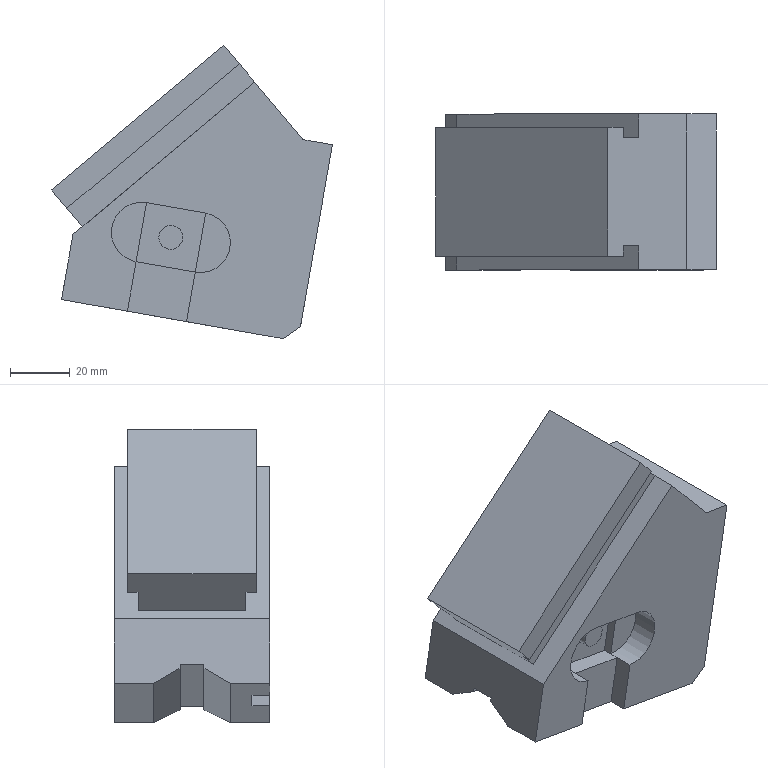Part | NX | features MAIN_BODY 2 | 1 solid | 38 faces | box 93.656 x 52 x 97.766 mm | volume 276638 mm3 | plane 35 | cylinder 2 | spline 1 | commonest cylinder face diameters 20 x2
STEP:
#1=CARTESIAN_POINT('',(264.879,130.,-23.774));
#2=VERTEX_POINT('',#1);
#3=CARTESIAN_POINT('',(297.078,130.,-29.451));
#4=VERTEX_POINT('',#3);
#5=CARTESIAN_POINT('',(223.218,130.,-16.428));
#6=DIRECTION('',(0.9848,0.,-0.1736));
#7=VECTOR('',#6,1000.);
#8=LINE('',#5,#7);
#9=EDGE_CURVE('',#2,#4,#8,.T.);
#10=ORIENTED_EDGE('',*,*,#9,.F.);
#11=CARTESIAN_POINT('',(264.879,136.,-23.774));
#12=VERTEX_POINT('',#11);
#13=CARTESIAN_POINT('',(264.879,182.,-23.774));
#14=DIRECTION('',(0.,-1.,0.));
#15=VECTOR('',#14,1000.);
#16=LINE('',#13,#15);
#17=EDGE_CURVE('',#12,#2,#16,.T.);
#18=ORIENTED_EDGE('',*,*,#17,.F.);
#19=CARTESIAN_POINT('',(245.183,136.,-20.301));
#20=VERTEX_POINT('',#19);
#21=CARTESIAN_POINT('',(223.218,136.,-16.428));
#22=DIRECTION('',(-0.9848,0.,0.1736));
#23=VECTOR('',#22,1000.);
#24=LINE('',#21,#23);
#25=EDGE_CURVE('',#12,#20,#24,.T.);
#26=ORIENTED_EDGE('',*,*,#25,.T.);
#27=CARTESIAN_POINT('',(245.183,130.,-20.301));
#28=VERTEX_POINT('',#27);
#29=CARTESIAN_POINT('',(245.183,182.,-20.301));
#30=DIRECTION('',(0.,-1.,0.));
#31=VECTOR('',#30,1000.);
#32=LINE('',#29,#31);
#33=EDGE_CURVE('',#20,#28,#32,.T.);
#34=ORIENTED_EDGE('',*,*,#33,.T.);
#35=CARTESIAN_POINT('',(223.218,130.,-16.428));
#36=VERTEX_POINT('',#35);
#37=CARTESIAN_POINT('',(223.218,130.,-16.428));
#38=DIRECTION('',(0.9848,0.,-0.1736));
#39=VECTOR('',#38,1000.);
#40=LINE('',#37,#39);
#41=EDGE_CURVE('',#36,#28,#40,.T.);
#42=ORIENTED_EDGE('',*,*,#41,.F.);
#43=CARTESIAN_POINT('',(223.218,143.01,-16.428));
#44=VERTEX_POINT('',#43);
#45=CARTESIAN_POINT('',(223.218,182.,-16.428));
#46=DIRECTION('',(0.,-1.,0.));
#47=VECTOR('',#46,1000.);
#48=LINE('',#45,#47);
#49=EDGE_CURVE('',#44,#36,#48,.T.);
#50=ORIENTED_EDGE('',*,*,#49,.F.);
#51=CARTESIAN_POINT('',(297.078,143.01,-29.451));
#52=VERTEX_POINT('',#51);
#53=CARTESIAN_POINT('',(223.218,143.01,-16.428));
#54=DIRECTION('',(-0.9848,0.,0.1736));
#55=VECTOR('',#54,1000.);
#56=LINE('',#53,#55);
#57=EDGE_CURVE('',#52,#44,#56,.T.);
#58=ORIENTED_EDGE('',*,*,#57,.F.);
#59=CARTESIAN_POINT('',(297.078,143.01,-29.451));
#60=DIRECTION('',(0.,1.,0.));
#61=VECTOR('',#60,1000.);
#62=LINE('',#59,#61);
#63=EDGE_CURVE('',#4,#52,#62,.T.);
#64=ORIENTED_EDGE('',*,*,#63,.F.);
#65=EDGE_LOOP('',(#10,#18,#26,#34,#42,#50,#58,#64));
#66=FACE_BOUND('',#65,.T.);
#67=CARTESIAN_POINT('',(223.218,182.,-16.428));
#68=DIRECTION('',(0.1736,0.,0.9848));
#69=DIRECTION('',(0.9848,0.,-0.1736));
#70=AXIS2_PLACEMENT_3D('',#67,#68,#69);
#71=PLANE('',#70);
#72=ADVANCED_FACE('',(#66),#71,.F.);
#73=CARTESIAN_POINT('',(313.55,130.,35.17));
#74=VERTEX_POINT('',#73);
#75=CARTESIAN_POINT('',(302.871,130.,-25.396));
#76=VERTEX_POINT('',#75);
#77=CARTESIAN_POINT('',(313.55,130.,35.17));
#78=DIRECTION('',(-0.1736,0.,-0.9848));
#79=VECTOR('',#78,1000.);
#80=LINE('',#77,#79);
#81=EDGE_CURVE('',#74,#76,#80,.T.);
#82=ORIENTED_EDGE('',*,*,#81,.F.);
#83=CARTESIAN_POINT('',(303.702,130.,36.906));
#84=VERTEX_POINT('',#83);
#85=CARTESIAN_POINT('',(303.702,130.,36.906));
#86=DIRECTION('',(0.9848,0.,-0.1736));
#87=VECTOR('',#86,1000.);
#88=LINE('',#85,#87);
#89=EDGE_CURVE('',#84,#74,#88,.T.);
#90=ORIENTED_EDGE('',*,*,#89,.F.);
#91=CARTESIAN_POINT('',(287.632,130.,56.058));
#92=VERTEX_POINT('',#91);
#93=CARTESIAN_POINT('',(287.632,130.,56.058));
#94=DIRECTION('',(0.6428,0.,-0.766));
#95=VECTOR('',#94,1000.);
#96=LINE('',#93,#95);
#97=EDGE_CURVE('',#92,#84,#96,.T.);
#98=ORIENTED_EDGE('',*,*,#97,.F.);
#99=CARTESIAN_POINT('',(227.033,130.,5.209));
#100=VERTEX_POINT('',#99);
#101=CARTESIAN_POINT('',(227.033,130.,5.209));
#102=DIRECTION('',(0.766,0.,0.6428));
#103=VECTOR('',#102,1000.);
#104=LINE('',#101,#103);
#105=EDGE_CURVE('',#100,#92,#104,.T.);
#106=ORIENTED_EDGE('',*,*,#105,.F.);
#107=CARTESIAN_POINT('',(227.033,130.,5.209));
#108=DIRECTION('',(-0.1736,0.,-0.9848));
#109=VECTOR('',#108,1000.);
#110=LINE('',#107,#109);
#111=EDGE_CURVE('',#100,#36,#110,.T.);
#112=ORIENTED_EDGE('',*,*,#111,.T.);
#113=ORIENTED_EDGE('',*,*,#41,.T.);
#114=CARTESIAN_POINT('',(248.091,130.,-3.808));
#115=VERTEX_POINT('',#114);
#116=CARTESIAN_POINT('',(251.564,130.,15.888));
#117=DIRECTION('',(-0.1736,0.,-0.9848));
#118=VECTOR('',#117,1000.);
#119=LINE('',#116,#118);
#120=EDGE_CURVE('',#115,#28,#119,.T.);
#121=ORIENTED_EDGE('',*,*,#120,.F.);
#122=CARTESIAN_POINT('',(251.564,130.,15.888));
#123=VERTEX_POINT('',#122);
#124=CARTESIAN_POINT('',(249.828,130.,6.04));
#125=DIRECTION('',(0.,-1.,0.));
#126=DIRECTION('',(0.9848,0.,0.1736));
#127=AXIS2_PLACEMENT_3D('',#124,#125,#126);
#128=CIRCLE('',#127,10.);
#129=EDGE_CURVE('',#123,#115,#128,.T.);
#130=ORIENTED_EDGE('',*,*,#129,.F.);
#131=CARTESIAN_POINT('',(271.26,130.,12.415));
#132=VERTEX_POINT('',#131);
#133=CARTESIAN_POINT('',(271.26,130.,12.415));
#134=DIRECTION('',(-0.9848,0.,0.1736));
#135=VECTOR('',#134,1000.);
#136=LINE('',#133,#135);
#137=EDGE_CURVE('',#132,#123,#136,.T.);
#138=ORIENTED_EDGE('',*,*,#137,.F.);
#139=CARTESIAN_POINT('',(267.787,130.,-7.281));
#140=VERTEX_POINT('',#139);
#141=CARTESIAN_POINT('',(269.524,130.,2.567));
#142=DIRECTION('',(0.,-1.,0.));
#143=DIRECTION('',(0.9848,0.,0.1736));
#144=AXIS2_PLACEMENT_3D('',#141,#142,#143);
#145=CIRCLE('',#144,10.);
#146=EDGE_CURVE('',#140,#132,#145,.T.);
#147=ORIENTED_EDGE('',*,*,#146,.F.);
#148=CARTESIAN_POINT('',(271.26,130.,12.415));
#149=DIRECTION('',(-0.1736,0.,-0.9848));
#150=VECTOR('',#149,1000.);
#151=LINE('',#148,#150);
#152=EDGE_CURVE('',#140,#2,#151,.T.);
#153=ORIENTED_EDGE('',*,*,#152,.T.);
#154=ORIENTED_EDGE('',*,*,#9,.T.);
#155=CARTESIAN_POINT('',(302.871,130.,-25.396));
#156=DIRECTION('',(-0.8192,0.,-0.5736));
#157=VECTOR('',#156,1000.);
#158=LINE('',#155,#157);
#159=EDGE_CURVE('',#76,#4,#158,.T.);
#160=ORIENTED_EDGE('',*,*,#159,.F.);
#161=EDGE_LOOP('',(#82,#90,#98,#106,#112,#113,#121,#130,#138,#147,#153,#154,#160));
#162=FACE_BOUND('',#161,.T.);
#163=CARTESIAN_POINT('',(223.218,130.,-16.428));
#164=DIRECTION('',(0.,1.,0.));
#165=DIRECTION('',(0.,0.,-1.));
#166=AXIS2_PLACEMENT_3D('',#163,#164,#165);
#167=PLANE('',#166);
#168=ADVANCED_FACE('',(#162),#167,.F.);
#169=CARTESIAN_POINT('',(267.787,136.,-7.281));
#170=VERTEX_POINT('',#169);
#171=CARTESIAN_POINT('',(248.091,136.,-3.808));
#172=VERTEX_POINT('',#171);
#173=CARTESIAN_POINT('',(267.787,136.,-7.281));
#174=DIRECTION('',(-0.9848,0.,0.1736));
#175=VECTOR('',#174,1000.);
#176=LINE('',#173,#175);
#177=EDGE_CURVE('',#170,#172,#176,.T.);
#178=ORIENTED_EDGE('',*,*,#177,.F.);
#179=CARTESIAN_POINT('',(267.787,139.,-7.281));
#180=VERTEX_POINT('',#179);
#181=CARTESIAN_POINT('',(267.787,139.,-7.281));
#182=DIRECTION('',(0.,-1.,0.));
#183=VECTOR('',#182,1000.);
#184=LINE('',#181,#183);
#185=EDGE_CURVE('',#180,#170,#184,.T.);
#186=ORIENTED_EDGE('',*,*,#185,.F.);
#187=CARTESIAN_POINT('',(267.787,142.,-7.281));
#188=VERTEX_POINT('',#187);
#189=CARTESIAN_POINT('',(267.787,142.,-7.281));
#190=DIRECTION('',(0.,-1.,0.));
#191=VECTOR('',#190,1000.);
#192=LINE('',#189,#191);
#193=EDGE_CURVE('',#188,#180,#192,.T.);
#194=ORIENTED_EDGE('',*,*,#193,.F.);
#195=CARTESIAN_POINT('',(248.091,142.,-3.808));
#196=VERTEX_POINT('',#195);
#197=CARTESIAN_POINT('',(267.787,142.,-7.281));
#198=DIRECTION('',(-0.9848,0.,0.1736));
#199=VECTOR('',#198,1000.);
#200=LINE('',#197,#199);
#201=EDGE_CURVE('',#188,#196,#200,.T.);
#202=ORIENTED_EDGE('',*,*,#201,.T.);
#203=CARTESIAN_POINT('',(248.091,139.,-3.808));
#204=VERTEX_POINT('',#203);
#205=CARTESIAN_POINT('',(248.091,142.,-3.808));
#206=DIRECTION('',(0.,-1.,0.));
#207=VECTOR('',#206,1000.);
#208=LINE('',#205,#207);
#209=EDGE_CURVE('',#196,#204,#208,.T.);
#210=ORIENTED_EDGE('',*,*,#209,.T.);
#211=CARTESIAN_POINT('',(248.091,139.,-3.808));
#212=DIRECTION('',(0.,-1.,0.));
#213=VECTOR('',#212,1000.);
#214=LINE('',#211,#213);
#215=EDGE_CURVE('',#204,#172,#214,.T.);
#216=ORIENTED_EDGE('',*,*,#215,.T.);
#217=EDGE_LOOP('',(#178,#186,#194,#202,#210,#216));
#218=FACE_BOUND('',#217,.T.);
#219=CARTESIAN_POINT('',(267.787,139.,-7.281));
#220=DIRECTION('',(-0.1736,0.,-0.9848));
#221=DIRECTION('',(-0.9848,0.,0.1736));
#222=AXIS2_PLACEMENT_3D('',#219,#220,#221);
#223=PLANE('',#222);
#224=ADVANCED_FACE('',(#218),#223,.F.);
#225=CARTESIAN_POINT('',(251.564,139.,15.888));
#226=VERTEX_POINT('',#225);
#227=CARTESIAN_POINT('',(249.828,139.,6.04));
#228=DIRECTION('',(0.1736,0.,0.9848));
#229=VECTOR('',#228,1000.);
#230=LINE('',#227,#229);
#231=EDGE_CURVE('',#204,#226,#230,.T.);
#232=ORIENTED_EDGE('',*,*,#231,.T.);
#233=CARTESIAN_POINT('',(249.828,139.,6.04));
#234=DIRECTION('',(0.,-1.,0.));
#235=DIRECTION('',(0.9848,0.,0.1736));
#236=AXIS2_PLACEMENT_3D('',#233,#234,#235);
#237=CIRCLE('',#236,10.);
#238=EDGE_CURVE('',#226,#204,#237,.T.);
#239=ORIENTED_EDGE('',*,*,#238,.T.);
#240=EDGE_LOOP('',(#232,#239));
#241=FACE_BOUND('',#240,.T.);
#242=CARTESIAN_POINT('',(249.828,139.,6.04));
#243=DIRECTION('',(0.,1.,0.));
#244=DIRECTION('',(0.,0.,-1.));
#245=AXIS2_PLACEMENT_3D('',#242,#243,#244);
#246=PLANE('',#245);
#247=ADVANCED_FACE('',(#241),#246,.F.);
#248=CARTESIAN_POINT('',(230.179,138.,7.849));
#249=VERTEX_POINT('',#248);
#250=CARTESIAN_POINT('',(230.179,174.,7.849));
#251=VERTEX_POINT('',#250);
#252=CARTESIAN_POINT('',(230.179,138.,7.849));
#253=DIRECTION('',(0.,1.,0.));
#254=VECTOR('',#253,1000.);
#255=LINE('',#252,#254);
#256=EDGE_CURVE('',#249,#251,#255,.T.);
#257=ORIENTED_EDGE('',*,*,#256,.T.);
#258=CARTESIAN_POINT('',(287.632,174.,56.058));
#259=VERTEX_POINT('',#258);
#260=CARTESIAN_POINT('',(230.179,174.,7.849));
#261=DIRECTION('',(0.766,0.,0.6428));
#262=VECTOR('',#261,1000.);
#263=LINE('',#260,#262);
#264=EDGE_CURVE('',#251,#259,#263,.T.);
#265=ORIENTED_EDGE('',*,*,#264,.T.);
#266=CARTESIAN_POINT('',(287.632,182.,56.058));
#267=VERTEX_POINT('',#266);
#268=CARTESIAN_POINT('',(287.632,182.,56.058));
#269=DIRECTION('',(0.,-1.,0.));
#270=VECTOR('',#269,1000.);
#271=LINE('',#268,#270);
#272=EDGE_CURVE('',#267,#259,#271,.T.);
#273=ORIENTED_EDGE('',*,*,#272,.F.);
#274=CARTESIAN_POINT('',(227.033,182.,5.209));
#275=VERTEX_POINT('',#274);
#276=CARTESIAN_POINT('',(227.033,182.,5.209));
#277=DIRECTION('',(0.766,0.,0.6428));
#278=VECTOR('',#277,1000.);
#279=LINE('',#276,#278);
#280=EDGE_CURVE('',#275,#267,#279,.T.);
#281=ORIENTED_EDGE('',*,*,#280,.F.);
#282=CARTESIAN_POINT('',(227.033,182.,5.209));
#283=DIRECTION('',(0.,-1.,0.));
#284=VECTOR('',#283,1000.);
#285=LINE('',#282,#284);
#286=EDGE_CURVE('',#275,#100,#285,.T.);
#287=ORIENTED_EDGE('',*,*,#286,.T.);
#288=ORIENTED_EDGE('',*,*,#105,.T.);
#289=CARTESIAN_POINT('',(287.632,138.,56.058));
#290=VERTEX_POINT('',#289);
#291=CARTESIAN_POINT('',(287.632,182.,56.058));
#292=DIRECTION('',(0.,-1.,0.));
#293=VECTOR('',#292,1000.);
#294=LINE('',#291,#293);
#295=EDGE_CURVE('',#290,#92,#294,.T.);
#296=ORIENTED_EDGE('',*,*,#295,.F.);
#297=CARTESIAN_POINT('',(230.179,138.,7.849));
#298=DIRECTION('',(0.766,0.,0.6428));
#299=VECTOR('',#298,1000.);
#300=LINE('',#297,#299);
#301=EDGE_CURVE('',#249,#290,#300,.T.);
#302=ORIENTED_EDGE('',*,*,#301,.F.);
#303=EDGE_LOOP('',(#257,#265,#273,#281,#287,#288,#296,#302));
#304=FACE_BOUND('',#303,.T.);
#305=CARTESIAN_POINT('',(227.033,182.,5.209));
#306=DIRECTION('',(-0.6428,0.,0.766));
#307=DIRECTION('',(0.766,0.,0.6428));
#308=AXIS2_PLACEMENT_3D('',#305,#306,#307);
#309=PLANE('',#308);
#310=ADVANCED_FACE('',(#304),#309,.T.);
#311=CARTESIAN_POINT('',(223.218,168.99,-16.428));
#312=VERTEX_POINT('',#311);
#313=CARTESIAN_POINT('',(297.078,168.99,-29.451));
#314=VERTEX_POINT('',#313);
#315=CARTESIAN_POINT('',(223.218,168.99,-16.428));
#316=DIRECTION('',(0.9848,0.,-0.1736));
#317=VECTOR('',#316,1000.);
#318=LINE('',#315,#317);
#319=EDGE_CURVE('',#312,#314,#318,.T.);
#320=ORIENTED_EDGE('',*,*,#319,.F.);
#321=CARTESIAN_POINT('',(223.218,182.,-16.428));
#322=VERTEX_POINT('',#321);
#323=CARTESIAN_POINT('',(223.218,182.,-16.428));
#324=DIRECTION('',(0.,-1.,0.));
#325=VECTOR('',#324,1000.);
#326=LINE('',#323,#325);
#327=EDGE_CURVE('',#322,#312,#326,.T.);
#328=ORIENTED_EDGE('',*,*,#327,.F.);
#329=CARTESIAN_POINT('',(297.078,182.,-29.451));
#330=VERTEX_POINT('',#329);
#331=CARTESIAN_POINT('',(223.218,182.,-16.428));
#332=DIRECTION('',(0.9848,0.,-0.1736));
#333=VECTOR('',#332,1000.);
#334=LINE('',#331,#333);
#335=EDGE_CURVE('',#322,#330,#334,.T.);
#336=ORIENTED_EDGE('',*,*,#335,.T.);
#337=CARTESIAN_POINT('',(297.078,182.,-29.451));
#338=DIRECTION('',(0.,1.,0.));
#339=VECTOR('',#338,1000.);
#340=LINE('',#337,#339);
#341=EDGE_CURVE('',#314,#330,#340,.T.);
#342=ORIENTED_EDGE('',*,*,#341,.F.);
#343=EDGE_LOOP('',(#320,#328,#336,#342));
#344=FACE_BOUND('',#343,.T.);
#345=CARTESIAN_POINT('',(223.218,182.,-16.428));
#346=DIRECTION('',(0.1736,0.,0.9848));
#347=DIRECTION('',(0.9848,0.,-0.1736));
#348=AXIS2_PLACEMENT_3D('',#345,#346,#347);
#349=PLANE('',#348);
#350=ADVANCED_FACE('',(#344),#349,.F.);
#351=CARTESIAN_POINT('',(224.346,160.,-10.027));
#352=VERTEX_POINT('',#351);
#353=CARTESIAN_POINT('',(224.119,160.,-11.316));
#354=VERTEX_POINT('',#353);
#355=CARTESIAN_POINT('',(224.346,160.,-10.027));
#356=DIRECTION('',(-0.1736,0.,-0.9848));
#357=VECTOR('',#356,1000.);
#358=LINE('',#355,#357);
#359=EDGE_CURVE('',#352,#354,#358,.T.);
#360=ORIENTED_EDGE('',*,*,#359,.F.);
#361=CARTESIAN_POINT('',(224.346,152.,-10.027));
#362=VERTEX_POINT('',#361);
#363=CARTESIAN_POINT('',(224.346,160.,-10.027));
#364=DIRECTION('',(0.,-1.,0.));
#365=VECTOR('',#364,1000.);
#366=LINE('',#363,#365);
#367=EDGE_CURVE('',#352,#362,#366,.T.);
#368=ORIENTED_EDGE('',*,*,#367,.T.);
#369=CARTESIAN_POINT('',(224.119,152.,-11.316));
#370=VERTEX_POINT('',#369);
#371=CARTESIAN_POINT('',(224.346,152.,-10.027));
#372=DIRECTION('',(-0.1736,0.,-0.9848));
#373=VECTOR('',#372,1000.);
#374=LINE('',#371,#373);
#375=EDGE_CURVE('',#362,#370,#374,.T.);
#376=ORIENTED_EDGE('',*,*,#375,.T.);
#377=CARTESIAN_POINT('',(223.218,143.01,-16.428));
#378=DIRECTION('',(-0.08682,-0.866,-0.4924));
#379=VECTOR('',#378,1000.);
#380=LINE('',#377,#379);
#381=EDGE_CURVE('',#370,#44,#380,.T.);
#382=ORIENTED_EDGE('',*,*,#381,.T.);
#383=ORIENTED_EDGE('',*,*,#49,.T.);
#384=ORIENTED_EDGE('',*,*,#111,.F.);
#385=ORIENTED_EDGE('',*,*,#286,.F.);
#386=CARTESIAN_POINT('',(227.033,182.,5.209));
#387=DIRECTION('',(-0.1736,0.,-0.9848));
#388=VECTOR('',#387,1000.);
#389=LINE('',#386,#388);
#390=EDGE_CURVE('',#275,#322,#389,.T.);
#391=ORIENTED_EDGE('',*,*,#390,.T.);
#392=ORIENTED_EDGE('',*,*,#327,.T.);
#393=CARTESIAN_POINT('',(223.218,168.99,-16.428));
#394=DIRECTION('',(0.08682,-0.866,0.4924));
#395=VECTOR('',#394,1000.);
#396=LINE('',#393,#395);
#397=EDGE_CURVE('',#312,#354,#396,.T.);
#398=ORIENTED_EDGE('',*,*,#397,.T.);
#399=EDGE_LOOP('',(#360,#368,#376,#382,#383,#384,#385,#391,#392,#398));
#400=FACE_BOUND('',#399,.T.);
#401=CARTESIAN_POINT('',(227.033,182.,5.209));
#402=DIRECTION('',(0.9848,0.,-0.1736));
#403=DIRECTION('',(-0.1736,0.,-0.9848));
#404=AXIS2_PLACEMENT_3D('',#401,#402,#403);
#405=PLANE('',#404);
#406=ADVANCED_FACE('',(#400),#405,.F.);
#407=CARTESIAN_POINT('',(302.904,152.,-25.208));
#408=VERTEX_POINT('',#407);
#409=CARTESIAN_POINT('',(302.871,151.67,-25.396));
#410=VERTEX_POINT('',#409);
#411=CARTESIAN_POINT('',(302.904,152.,-25.208));
#412=DIRECTION('',(-0.08682,-0.866,-0.4924));
#413=VECTOR('',#412,1000.);
#414=LINE('',#411,#413);
#415=EDGE_CURVE('',#408,#410,#414,.T.);
#416=ORIENTED_EDGE('',*,*,#415,.F.);
#417=CARTESIAN_POINT('',(303.131,152.,-23.918));
#418=VERTEX_POINT('',#417);
#419=CARTESIAN_POINT('',(303.131,152.,-23.918));
#420=DIRECTION('',(-0.1736,0.,-0.9848));
#421=VECTOR('',#420,1000.);
#422=LINE('',#419,#421);
#423=EDGE_CURVE('',#418,#408,#422,.T.);
#424=ORIENTED_EDGE('',*,*,#423,.F.);
#425=CARTESIAN_POINT('',(303.131,160.,-23.918));
#426=VERTEX_POINT('',#425);
#427=CARTESIAN_POINT('',(303.131,160.,-23.918));
#428=DIRECTION('',(0.,-1.,0.));
#429=VECTOR('',#428,1000.);
#430=LINE('',#427,#429);
#431=EDGE_CURVE('',#426,#418,#430,.T.);
#432=ORIENTED_EDGE('',*,*,#431,.F.);
#433=CARTESIAN_POINT('',(302.904,160.,-25.208));
#434=VERTEX_POINT('',#433);
#435=CARTESIAN_POINT('',(303.131,160.,-23.918));
#436=DIRECTION('',(-0.1736,0.,-0.9848));
#437=VECTOR('',#436,1000.);
#438=LINE('',#435,#437);
#439=EDGE_CURVE('',#426,#434,#438,.T.);
#440=ORIENTED_EDGE('',*,*,#439,.T.);
#441=CARTESIAN_POINT('',(302.871,160.33,-25.396));
#442=VERTEX_POINT('',#441);
#443=CARTESIAN_POINT('',(302.002,168.99,-30.32));
#444=DIRECTION('',(0.08682,-0.866,0.4924));
#445=VECTOR('',#444,1000.);
#446=LINE('',#443,#445);
#447=EDGE_CURVE('',#442,#434,#446,.T.);
#448=ORIENTED_EDGE('',*,*,#447,.F.);
#449=CARTESIAN_POINT('',(302.871,182.,-25.396));
#450=VERTEX_POINT('',#449);
#451=CARTESIAN_POINT('',(302.871,168.99,-25.396));
#452=DIRECTION('',(0.,-1.,0.));
#453=VECTOR('',#452,1000.);
#454=LINE('',#451,#453);
#455=EDGE_CURVE('',#450,#442,#454,.T.);
#456=ORIENTED_EDGE('',*,*,#455,.F.);
#457=CARTESIAN_POINT('',(313.55,182.,35.17));
#458=VERTEX_POINT('',#457);
#459=CARTESIAN_POINT('',(313.55,182.,35.17));
#460=DIRECTION('',(-0.1736,0.,-0.9848));
#461=VECTOR('',#460,1000.);
#462=LINE('',#459,#461);
#463=EDGE_CURVE('',#458,#450,#462,.T.);
#464=ORIENTED_EDGE('',*,*,#463,.F.);
#465=CARTESIAN_POINT('',(313.55,182.,35.17));
#466=DIRECTION('',(0.,-1.,0.));
#467=VECTOR('',#466,1000.);
#468=LINE('',#465,#467);
#469=EDGE_CURVE('',#458,#74,#468,.T.);
#470=ORIENTED_EDGE('',*,*,#469,.T.);
#471=ORIENTED_EDGE('',*,*,#81,.T.);
#472=CARTESIAN_POINT('',(302.871,130.,-25.396));
#473=DIRECTION('',(0.,-1.,0.));
#474=VECTOR('',#473,1000.);
#475=LINE('',#472,#474);
#476=EDGE_CURVE('',#410,#76,#475,.T.);
#477=ORIENTED_EDGE('',*,*,#476,.F.);
#478=EDGE_LOOP('',(#416,#424,#432,#440,#448,#456,#464,#470,#471,#477));
#479=FACE_BOUND('',#478,.T.);
#480=CARTESIAN_POINT('',(313.55,182.,35.17));
#481=DIRECTION('',(0.9848,0.,-0.1736));
#482=DIRECTION('',(-0.1736,0.,-0.9848));
#483=AXIS2_PLACEMENT_3D('',#480,#481,#482);
#484=PLANE('',#483);
#485=ADVANCED_FACE('',(#479),#484,.T.);
#486=ORIENTED_EDGE('',*,*,#89,.T.);
#487=ORIENTED_EDGE('',*,*,#469,.F.);
#488=CARTESIAN_POINT('',(303.702,182.,36.906));
#489=VERTEX_POINT('',#488);
#490=CARTESIAN_POINT('',(303.702,182.,36.906));
#491=DIRECTION('',(0.9848,0.,-0.1736));
#492=VECTOR('',#491,1000.);
#493=LINE('',#490,#492);
#494=EDGE_CURVE('',#489,#458,#493,.T.);
#495=ORIENTED_EDGE('',*,*,#494,.F.);
#496=CARTESIAN_POINT('',(303.702,182.,36.906));
#497=DIRECTION('',(0.,-1.,0.));
#498=VECTOR('',#497,1000.);
#499=LINE('',#496,#498);
#500=EDGE_CURVE('',#489,#84,#499,.T.);
#501=ORIENTED_EDGE('',*,*,#500,.T.);
#502=EDGE_LOOP('',(#486,#487,#495,#501));
#503=FACE_BOUND('',#502,.T.);
#504=CARTESIAN_POINT('',(303.702,182.,36.906));
#505=DIRECTION('',(0.1736,0.,0.9848));
#506=DIRECTION('',(0.9848,0.,-0.1736));
#507=AXIS2_PLACEMENT_3D('',#504,#505,#506);
#508=PLANE('',#507);
#509=ADVANCED_FACE('',(#503),#508,.T.);
#510=ORIENTED_EDGE('',*,*,#97,.T.);
#511=ORIENTED_EDGE('',*,*,#500,.F.);
#512=CARTESIAN_POINT('',(287.632,182.,56.058));
#513=DIRECTION('',(0.6428,0.,-0.766));
#514=VECTOR('',#513,1000.);
#515=LINE('',#512,#514);
#516=EDGE_CURVE('',#267,#489,#515,.T.);
#517=ORIENTED_EDGE('',*,*,#516,.F.);
#518=ORIENTED_EDGE('',*,*,#272,.T.);
#519=CARTESIAN_POINT('',(282.49,174.,62.186));
#520=VERTEX_POINT('',#519);
#521=CARTESIAN_POINT('',(282.49,174.,62.186));
#522=DIRECTION('',(0.6428,0.,-0.766));
#523=VECTOR('',#522,1000.);
#524=LINE('',#521,#523);
#525=EDGE_CURVE('',#520,#259,#524,.T.);
#526=ORIENTED_EDGE('',*,*,#525,.F.);
#527=CARTESIAN_POINT('',(282.49,177.5,62.186));
#528=VERTEX_POINT('',#527);
#529=CARTESIAN_POINT('',(282.49,134.5,62.186));
#530=DIRECTION('',(0.,1.,0.));
#531=VECTOR('',#530,1000.);
#532=LINE('',#529,#531);
#533=EDGE_CURVE('',#520,#528,#532,.T.);
#534=ORIENTED_EDGE('',*,*,#533,.T.);
#535=CARTESIAN_POINT('',(277.348,177.5,68.314));
#536=VERTEX_POINT('',#535);
#537=CARTESIAN_POINT('',(277.348,177.5,68.314));
#538=DIRECTION('',(0.6428,0.,-0.766));
#539=VECTOR('',#538,1000.);
#540=LINE('',#537,#539);
#541=EDGE_CURVE('',#536,#528,#540,.T.);
#542=ORIENTED_EDGE('',*,*,#541,.F.);
#543=CARTESIAN_POINT('',(277.348,134.5,68.314));
#544=VERTEX_POINT('',#543);
#545=CARTESIAN_POINT('',(277.348,134.5,68.314));
#546=DIRECTION('',(0.,1.,0.));
#547=VECTOR('',#546,1000.);
#548=LINE('',#545,#547);
#549=EDGE_CURVE('',#544,#536,#548,.T.);
#550=ORIENTED_EDGE('',*,*,#549,.F.);
#551=CARTESIAN_POINT('',(282.49,134.5,62.186));
#552=VERTEX_POINT('',#551);
#553=CARTESIAN_POINT('',(277.348,134.5,68.314));
#554=DIRECTION('',(0.6428,0.,-0.766));
#555=VECTOR('',#554,1000.);
#556=LINE('',#553,#555);
#557=EDGE_CURVE('',#544,#552,#556,.T.);
#558=ORIENTED_EDGE('',*,*,#557,.T.);
#559=CARTESIAN_POINT('',(282.49,138.,62.186));
#560=VERTEX_POINT('',#559);
#561=CARTESIAN_POINT('',(282.49,134.5,62.186));
#562=DIRECTION('',(0.,1.,0.));
#563=VECTOR('',#562,1000.);
#564=LINE('',#561,#563);
#565=EDGE_CURVE('',#552,#560,#564,.T.);
#566=ORIENTED_EDGE('',*,*,#565,.T.);
#567=CARTESIAN_POINT('',(282.49,138.,62.186));
#568=DIRECTION('',(0.6428,0.,-0.766));
#569=VECTOR('',#568,1000.);
#570=LINE('',#567,#569);
#571=EDGE_CURVE('',#560,#290,#570,.T.);
#572=ORIENTED_EDGE('',*,*,#571,.T.);
#573=ORIENTED_EDGE('',*,*,#295,.T.);
#574=EDGE_LOOP('',(#510,#511,#517,#518,#526,#534,#542,#550,#558,#566,#572,#573));
#575=FACE_BOUND('',#574,.T.);
#576=CARTESIAN_POINT('',(287.632,182.,56.058));
#577=DIRECTION('',(0.766,0.,0.6428));
#578=DIRECTION('',(0.6428,0.,-0.766));
#579=AXIS2_PLACEMENT_3D('',#576,#577,#578);
#580=PLANE('',#579);
#581=ADVANCED_FACE('',(#575),#580,.T.);
#582=ORIENTED_EDGE('',*,*,#335,.F.);
#583=ORIENTED_EDGE('',*,*,#390,.F.);
#584=ORIENTED_EDGE('',*,*,#280,.T.);
#585=ORIENTED_EDGE('',*,*,#516,.T.);
#586=ORIENTED_EDGE('',*,*,#494,.T.);
#587=ORIENTED_EDGE('',*,*,#463,.T.);
#588=CARTESIAN_POINT('',(253.636,182.,-59.87));
#589=DIRECTION('',(0.8192,0.,0.5736));
#590=VECTOR('',#589,1000.);
#591=LINE('',#588,#590);
#592=EDGE_CURVE('',#330,#450,#591,.T.);
#593=ORIENTED_EDGE('',*,*,#592,.F.);
#594=EDGE_LOOP('',(#582,#583,#584,#585,#586,#587,#593));
#595=FACE_BOUND('',#594,.T.);
#596=CARTESIAN_POINT('',(223.218,182.,-16.428));
#597=DIRECTION('',(0.,1.,0.));
#598=DIRECTION('',(0.,0.,-1.));
#599=AXIS2_PLACEMENT_3D('',#596,#597,#598);
#600=PLANE('',#599);
#601=ADVANCED_FACE('',(#595),#600,.T.);
#602=ORIENTED_EDGE('',*,*,#447,.T.);
#603=CARTESIAN_POINT('',(302.904,160.,-25.208));
#604=DIRECTION('',(-0.9848,0.,0.1736));
#605=VECTOR('',#604,1000.);
#606=LINE('',#603,#605);
#607=EDGE_CURVE('',#434,#354,#606,.T.);
#608=ORIENTED_EDGE('',*,*,#607,.T.);
#609=ORIENTED_EDGE('',*,*,#397,.F.);
#610=ORIENTED_EDGE('',*,*,#319,.T.);
#611=CARTESIAN_POINT('',(294.174,173.332,-31.485));
#612=DIRECTION('',(-0.5181,0.7746,-0.3628));
#613=VECTOR('',#612,1000.);
#614=LINE('',#611,#613);
#615=EDGE_CURVE('',#442,#314,#614,.T.);
#616=ORIENTED_EDGE('',*,*,#615,.F.);
#617=EDGE_LOOP('',(#602,#608,#609,#610,#616));
#618=FACE_BOUND('',#617,.T.);
#619=CARTESIAN_POINT('',(302.002,168.99,-30.32));
#620=DIRECTION('',(0.1504,0.5,0.8529));
#621=DIRECTION('',(0.,0.8627,-0.5058));
#622=AXIS2_PLACEMENT_3D('',#619,#620,#621);
#623=PLANE('',#622);
#624=ADVANCED_FACE('',(#618),#623,.F.);
#625=ORIENTED_EDGE('',*,*,#57,.T.);
#626=ORIENTED_EDGE('',*,*,#381,.F.);
#627=CARTESIAN_POINT('',(302.904,152.,-25.208));
#628=DIRECTION('',(-0.9848,0.,0.1736));
#629=VECTOR('',#628,1000.);
#630=LINE('',#627,#629);
#631=EDGE_CURVE('',#408,#370,#630,.T.);
#632=ORIENTED_EDGE('',*,*,#631,.F.);
#633=ORIENTED_EDGE('',*,*,#415,.T.);
#634=CARTESIAN_POINT('',(315.042,169.868,-16.873));
#635=DIRECTION('',(0.5181,0.7746,0.3628));
#636=VECTOR('',#635,1000.);
#637=LINE('',#634,#636);
#638=EDGE_CURVE('',#52,#410,#637,.T.);
#639=ORIENTED_EDGE('',*,*,#638,.F.);
#640=EDGE_LOOP('',(#625,#626,#632,#633,#639));
#641=FACE_BOUND('',#640,.T.);
#642=CARTESIAN_POINT('',(302.002,143.01,-30.32));
#643=DIRECTION('',(0.1504,-0.5,0.8529));
#644=DIRECTION('',(0.,0.8627,0.5058));
#645=AXIS2_PLACEMENT_3D('',#642,#643,#644);
#646=PLANE('',#645);
#647=ADVANCED_FACE('',(#641),#646,.F.);
#648=ORIENTED_EDGE('',*,*,#359,.T.);
#649=ORIENTED_EDGE('',*,*,#607,.F.);
#650=ORIENTED_EDGE('',*,*,#439,.F.);
#651=CARTESIAN_POINT('',(303.131,160.,-23.918));
#652=DIRECTION('',(-0.9848,0.,0.1736));
#653=VECTOR('',#652,1000.);
#654=LINE('',#651,#653);
#655=EDGE_CURVE('',#426,#352,#654,.T.);
#656=ORIENTED_EDGE('',*,*,#655,.T.);
#657=EDGE_LOOP('',(#648,#649,#650,#656));
#658=FACE_BOUND('',#657,.T.);
#659=CARTESIAN_POINT('',(303.131,160.,-23.918));
#660=DIRECTION('',(0.,-1.,0.));
#661=DIRECTION('',(0.,0.,1.));
#662=AXIS2_PLACEMENT_3D('',#659,#660,#661);
#663=PLANE('',#662);
#664=ADVANCED_FACE('',(#658),#663,.T.);
#665=ORIENTED_EDGE('',*,*,#367,.F.);
#666=ORIENTED_EDGE('',*,*,#655,.F.);
#667=ORIENTED_EDGE('',*,*,#431,.T.);
#668=CARTESIAN_POINT('',(303.131,152.,-23.918));
#669=DIRECTION('',(-0.9848,0.,0.1736));
#670=VECTOR('',#669,1000.);
#671=LINE('',#668,#670);
#672=EDGE_CURVE('',#418,#362,#671,.T.);
#673=ORIENTED_EDGE('',*,*,#672,.T.);
#674=EDGE_LOOP('',(#665,#666,#667,#673));
#675=FACE_BOUND('',#674,.T.);
#676=CARTESIAN_POINT('',(303.131,160.,-23.918));
#677=DIRECTION('',(0.1736,0.,0.9848));
#678=DIRECTION('',(0.9848,0.,-0.1736));
#679=AXIS2_PLACEMENT_3D('',#676,#677,#678);
#680=PLANE('',#679);
#681=ADVANCED_FACE('',(#675),#680,.F.);
#682=ORIENTED_EDGE('',*,*,#375,.F.);
#683=ORIENTED_EDGE('',*,*,#672,.F.);
#684=ORIENTED_EDGE('',*,*,#423,.T.);
#685=ORIENTED_EDGE('',*,*,#631,.T.);
#686=EDGE_LOOP('',(#682,#683,#684,#685));
#687=FACE_BOUND('',#686,.T.);
#688=CARTESIAN_POINT('',(303.131,152.,-23.918));
#689=DIRECTION('',(0.,-1.,0.));
#690=DIRECTION('',(0.,0.,1.));
#691=AXIS2_PLACEMENT_3D('',#688,#689,#690);
#692=PLANE('',#691);
#693=ADVANCED_FACE('',(#687),#692,.F.);
#694=CARTESIAN_POINT('',(225.037,174.,13.977));
#695=VERTEX_POINT('',#694);
#696=CARTESIAN_POINT('',(225.037,174.,13.977));
#697=DIRECTION('',(0.6428,0.,-0.766));
#698=VECTOR('',#697,1000.);
#699=LINE('',#696,#698);
#700=EDGE_CURVE('',#695,#251,#699,.T.);
#701=ORIENTED_EDGE('',*,*,#700,.T.);
#702=ORIENTED_EDGE('',*,*,#256,.F.);
#703=CARTESIAN_POINT('',(225.037,138.,13.977));
#704=VERTEX_POINT('',#703);
#705=CARTESIAN_POINT('',(225.037,138.,13.977));
#706=DIRECTION('',(0.6428,0.,-0.766));
#707=VECTOR('',#706,1000.);
#708=LINE('',#705,#707);
#709=EDGE_CURVE('',#704,#249,#708,.T.);
#710=ORIENTED_EDGE('',*,*,#709,.F.);
#711=CARTESIAN_POINT('',(225.037,134.5,13.977));
#712=VERTEX_POINT('',#711);
#713=CARTESIAN_POINT('',(225.037,134.5,13.977));
#714=DIRECTION('',(0.,1.,0.));
#715=VECTOR('',#714,1000.);
#716=LINE('',#713,#715);
#717=EDGE_CURVE('',#712,#704,#716,.T.);
#718=ORIENTED_EDGE('',*,*,#717,.F.);
#719=CARTESIAN_POINT('',(219.894,134.5,20.105));
#720=VERTEX_POINT('',#719);
#721=CARTESIAN_POINT('',(219.894,134.5,20.105));
#722=DIRECTION('',(0.6428,0.,-0.766));
#723=VECTOR('',#722,1000.);
#724=LINE('',#721,#723);
#725=EDGE_CURVE('',#720,#712,#724,.T.);
#726=ORIENTED_EDGE('',*,*,#725,.F.);
#727=CARTESIAN_POINT('',(219.894,177.5,20.105));
#728=VERTEX_POINT('',#727);
#729=CARTESIAN_POINT('',(219.894,134.5,20.105));
#730=DIRECTION('',(0.,1.,0.));
#731=VECTOR('',#730,1000.);
#732=LINE('',#729,#731);
#733=EDGE_CURVE('',#720,#728,#732,.T.);
#734=ORIENTED_EDGE('',*,*,#733,.T.);
#735=CARTESIAN_POINT('',(225.037,177.5,13.977));
#736=VERTEX_POINT('',#735);
#737=CARTESIAN_POINT('',(219.894,177.5,20.105));
#738=DIRECTION('',(0.6428,0.,-0.766));
#739=VECTOR('',#738,1000.);
#740=LINE('',#737,#739);
#741=EDGE_CURVE('',#728,#736,#740,.T.);
#742=ORIENTED_EDGE('',*,*,#741,.T.);
#743=CARTESIAN_POINT('',(225.037,134.5,13.977));
#744=DIRECTION('',(0.,1.,0.));
#745=VECTOR('',#744,1000.);
#746=LINE('',#743,#745);
#747=EDGE_CURVE('',#695,#736,#746,.T.);
#748=ORIENTED_EDGE('',*,*,#747,.F.);
#749=EDGE_LOOP('',(#701,#702,#710,#718,#726,#734,#742,#748));
#750=FACE_BOUND('',#749,.T.);
#751=CARTESIAN_POINT('',(225.037,138.,13.977));
#752=DIRECTION('',(-0.766,0.,-0.6428));
#753=DIRECTION('',(-0.6428,0.,0.766));
#754=AXIS2_PLACEMENT_3D('',#751,#752,#753);
#755=PLANE('',#754);
#756=ADVANCED_FACE('',(#750),#755,.T.);
#757=CARTESIAN_POINT('',(282.49,138.,62.186));
#758=DIRECTION('',(-0.766,0.,-0.6428));
#759=VECTOR('',#758,1000.);
#760=LINE('',#757,#759);
#761=EDGE_CURVE('',#560,#704,#760,.T.);
#762=ORIENTED_EDGE('',*,*,#761,.T.);
#763=ORIENTED_EDGE('',*,*,#709,.T.);
#764=ORIENTED_EDGE('',*,*,#301,.T.);
#765=ORIENTED_EDGE('',*,*,#571,.F.);
#766=EDGE_LOOP('',(#762,#763,#764,#765));
#767=FACE_BOUND('',#766,.T.);
#768=CARTESIAN_POINT('',(282.49,138.,62.186));
#769=DIRECTION('',(0.,1.,0.));
#770=DIRECTION('',(0.,0.,-1.));
#771=AXIS2_PLACEMENT_3D('',#768,#769,#770);
#772=PLANE('',#771);
#773=ADVANCED_FACE('',(#767),#772,.F.);
#774=CARTESIAN_POINT('',(282.49,174.,62.186));
#775=DIRECTION('',(-0.766,0.,-0.6428));
#776=VECTOR('',#775,1000.);
#777=LINE('',#774,#776);
#778=EDGE_CURVE('',#520,#695,#777,.T.);
#779=ORIENTED_EDGE('',*,*,#778,.F.);
#780=ORIENTED_EDGE('',*,*,#525,.T.);
#781=ORIENTED_EDGE('',*,*,#264,.F.);
#782=ORIENTED_EDGE('',*,*,#700,.F.);
#783=EDGE_LOOP('',(#779,#780,#781,#782));
#784=FACE_BOUND('',#783,.T.);
#785=CARTESIAN_POINT('',(282.49,174.,62.186));
#786=DIRECTION('',(0.,1.,0.));
#787=DIRECTION('',(0.,0.,-1.));
#788=AXIS2_PLACEMENT_3D('',#785,#786,#787);
#789=PLANE('',#788);
#790=ADVANCED_FACE('',(#784),#789,.T.);
#791=ORIENTED_EDGE('',*,*,#565,.F.);
#792=CARTESIAN_POINT('',(282.49,134.5,62.186));
#793=DIRECTION('',(-0.766,0.,-0.6428));
#794=VECTOR('',#793,1000.);
#795=LINE('',#792,#794);
#796=EDGE_CURVE('',#552,#712,#795,.T.);
#797=ORIENTED_EDGE('',*,*,#796,.T.);
#798=ORIENTED_EDGE('',*,*,#717,.T.);
#799=ORIENTED_EDGE('',*,*,#761,.F.);
#800=EDGE_LOOP('',(#791,#797,#798,#799));
#801=FACE_BOUND('',#800,.T.);
#802=CARTESIAN_POINT('',(282.49,134.5,62.186));
#803=DIRECTION('',(-0.6428,0.,0.766));
#804=DIRECTION('',(0.766,0.,0.6428));
#805=AXIS2_PLACEMENT_3D('',#802,#803,#804);
#806=PLANE('',#805);
#807=ADVANCED_FACE('',(#801),#806,.F.);
#808=ORIENTED_EDGE('',*,*,#778,.T.);
#809=ORIENTED_EDGE('',*,*,#747,.T.);
#810=CARTESIAN_POINT('',(282.49,177.5,62.186));
#811=DIRECTION('',(-0.766,0.,-0.6428));
#812=VECTOR('',#811,1000.);
#813=LINE('',#810,#812);
#814=EDGE_CURVE('',#528,#736,#813,.T.);
#815=ORIENTED_EDGE('',*,*,#814,.F.);
#816=ORIENTED_EDGE('',*,*,#533,.F.);
#817=EDGE_LOOP('',(#808,#809,#815,#816));
#818=FACE_BOUND('',#817,.T.);
#819=CARTESIAN_POINT('',(282.49,134.5,62.186));
#820=DIRECTION('',(-0.6428,0.,0.766));
#821=DIRECTION('',(0.766,0.,0.6428));
#822=AXIS2_PLACEMENT_3D('',#819,#820,#821);
#823=PLANE('',#822);
#824=ADVANCED_FACE('',(#818),#823,.F.);
#825=CARTESIAN_POINT('',(219.894,177.5,20.105));
#826=DIRECTION('',(0.766,0.,0.6428));
#827=VECTOR('',#826,1000.);
#828=LINE('',#825,#827);
#829=EDGE_CURVE('',#728,#536,#828,.T.);
#830=ORIENTED_EDGE('',*,*,#829,.F.);
#831=ORIENTED_EDGE('',*,*,#733,.F.);
#832=CARTESIAN_POINT('',(219.894,134.5,20.105));
#833=DIRECTION('',(0.766,0.,0.6428));
#834=VECTOR('',#833,1000.);
#835=LINE('',#832,#834);
#836=EDGE_CURVE('',#720,#544,#835,.T.);
#837=ORIENTED_EDGE('',*,*,#836,.T.);
#838=ORIENTED_EDGE('',*,*,#549,.T.);
#839=EDGE_LOOP('',(#830,#831,#837,#838));
#840=FACE_BOUND('',#839,.T.);
#841=CARTESIAN_POINT('',(219.894,134.5,20.105));
#842=DIRECTION('',(0.6428,0.,-0.766));
#843=DIRECTION('',(-0.766,0.,-0.6428));
#844=AXIS2_PLACEMENT_3D('',#841,#842,#843);
#845=PLANE('',#844);
#846=ADVANCED_FACE('',(#840),#845,.F.);
#847=ORIENTED_EDGE('',*,*,#796,.F.);
#848=ORIENTED_EDGE('',*,*,#557,.F.);
#849=ORIENTED_EDGE('',*,*,#836,.F.);
#850=ORIENTED_EDGE('',*,*,#725,.T.);
#851=EDGE_LOOP('',(#847,#848,#849,#850));
#852=FACE_BOUND('',#851,.T.);
#853=CARTESIAN_POINT('',(225.037,134.5,13.977));
#854=DIRECTION('',(0.,1.,0.));
#855=DIRECTION('',(0.,0.,-1.));
#856=AXIS2_PLACEMENT_3D('',#853,#854,#855);
#857=PLANE('',#856);
#858=ADVANCED_FACE('',(#852),#857,.F.);
#859=ORIENTED_EDGE('',*,*,#814,.T.);
#860=ORIENTED_EDGE('',*,*,#741,.F.);
#861=ORIENTED_EDGE('',*,*,#829,.T.);
#862=ORIENTED_EDGE('',*,*,#541,.T.);
#863=EDGE_LOOP('',(#859,#860,#861,#862));
#864=FACE_BOUND('',#863,.T.);
#865=CARTESIAN_POINT('',(225.037,177.5,13.977));
#866=DIRECTION('',(0.,1.,0.));
#867=DIRECTION('',(0.,0.,-1.));
#868=AXIS2_PLACEMENT_3D('',#865,#866,#867);
#869=PLANE('',#868);
#870=ADVANCED_FACE('',(#864),#869,.T.);
#871=ORIENTED_EDGE('',*,*,#129,.T.);
#872=CARTESIAN_POINT('',(248.091,139.,-3.808));
#873=DIRECTION('',(0.,-1.,0.));
#874=VECTOR('',#873,1000.);
#875=LINE('',#872,#874);
#876=EDGE_CURVE('',#172,#115,#875,.T.);
#877=ORIENTED_EDGE('',*,*,#876,.F.);
#878=ORIENTED_EDGE('',*,*,#215,.F.);
#879=ORIENTED_EDGE('',*,*,#238,.F.);
#880=CARTESIAN_POINT('',(251.564,139.,15.888));
#881=DIRECTION('',(0.,-1.,0.));
#882=VECTOR('',#881,1000.);
#883=LINE('',#880,#882);
#884=EDGE_CURVE('',#226,#123,#883,.T.);
#885=ORIENTED_EDGE('',*,*,#884,.T.);
#886=EDGE_LOOP('',(#871,#877,#878,#879,#885));
#887=FACE_BOUND('',#886,.T.);
#888=CARTESIAN_POINT('',(249.828,139.,6.04));
#889=DIRECTION('',(0.,-1.,0.));
#890=DIRECTION('',(0.,0.,1.));
#891=AXIS2_PLACEMENT_3D('',#888,#889,#890);
#892=CYLINDRICAL_SURFACE('',#891,10.);
#893=ADVANCED_FACE('',(#887),#892,.F.);
#894=ORIENTED_EDGE('',*,*,#137,.T.);
#895=ORIENTED_EDGE('',*,*,#884,.F.);
#896=CARTESIAN_POINT('',(251.564,142.,15.888));
#897=VERTEX_POINT('',#896);
#898=CARTESIAN_POINT('',(251.564,130.,15.888));
#899=DIRECTION('',(0.,1.,0.));
#900=VECTOR('',#899,1000.);
#901=LINE('',#898,#900);
#902=EDGE_CURVE('',#226,#897,#901,.T.);
#903=ORIENTED_EDGE('',*,*,#902,.T.);
#904=CARTESIAN_POINT('',(271.26,142.,12.415));
#905=VERTEX_POINT('',#904);
#906=CARTESIAN_POINT('',(271.26,142.,12.415));
#907=DIRECTION('',(-0.9848,0.,0.1736));
#908=VECTOR('',#907,1000.);
#909=LINE('',#906,#908);
#910=EDGE_CURVE('',#905,#897,#909,.T.);
#911=ORIENTED_EDGE('',*,*,#910,.F.);
#912=CARTESIAN_POINT('',(271.26,139.,12.415));
#913=VERTEX_POINT('',#912);
#914=CARTESIAN_POINT('',(271.26,130.,12.415));
#915=DIRECTION('',(0.,1.,0.));
#916=VECTOR('',#915,1000.);
#917=LINE('',#914,#916);
#918=EDGE_CURVE('',#913,#905,#917,.T.);
#919=ORIENTED_EDGE('',*,*,#918,.F.);
#920=CARTESIAN_POINT('',(271.26,139.,12.415));
#921=DIRECTION('',(0.,-1.,0.));
#922=VECTOR('',#921,1000.);
#923=LINE('',#920,#922);
#924=EDGE_CURVE('',#913,#132,#923,.T.);
#925=ORIENTED_EDGE('',*,*,#924,.T.);
#926=EDGE_LOOP('',(#894,#895,#903,#911,#919,#925));
#927=FACE_BOUND('',#926,.T.);
#928=CARTESIAN_POINT('',(271.26,139.,12.415));
#929=DIRECTION('',(-0.1736,0.,-0.9848));
#930=DIRECTION('',(-0.9848,0.,0.1736));
#931=AXIS2_PLACEMENT_3D('',#928,#929,#930);
#932=PLANE('',#931);
#933=ADVANCED_FACE('',(#927),#932,.T.);
#934=ORIENTED_EDGE('',*,*,#146,.T.);
#935=ORIENTED_EDGE('',*,*,#924,.F.);
#936=CARTESIAN_POINT('',(269.524,139.,2.567));
#937=DIRECTION('',(0.,-1.,0.));
#938=DIRECTION('',(0.9848,0.,0.1736));
#939=AXIS2_PLACEMENT_3D('',#936,#937,#938);
#940=CIRCLE('',#939,10.);
#941=EDGE_CURVE('',#180,#913,#940,.T.);
#942=ORIENTED_EDGE('',*,*,#941,.F.);
#943=ORIENTED_EDGE('',*,*,#185,.T.);
#944=CARTESIAN_POINT('',(267.787,139.,-7.281));
#945=DIRECTION('',(0.,-1.,0.));
#946=VECTOR('',#945,1000.);
#947=LINE('',#944,#946);
#948=EDGE_CURVE('',#170,#140,#947,.T.);
#949=ORIENTED_EDGE('',*,*,#948,.T.);
#950=EDGE_LOOP('',(#934,#935,#942,#943,#949));
#951=FACE_BOUND('',#950,.T.);
#952=CARTESIAN_POINT('',(269.524,139.,2.567));
#953=DIRECTION('',(0.,-1.,0.));
#954=DIRECTION('',(0.,0.,1.));
#955=AXIS2_PLACEMENT_3D('',#952,#953,#954);
#956=CYLINDRICAL_SURFACE('',#955,10.);
#957=ADVANCED_FACE('',(#951),#956,.F.);
#958=ORIENTED_EDGE('',*,*,#941,.T.);
#959=CARTESIAN_POINT('',(269.524,139.,2.567));
#960=DIRECTION('',(0.1736,0.,0.9848));
#961=VECTOR('',#960,1000.);
#962=LINE('',#959,#961);
#963=EDGE_CURVE('',#180,#913,#962,.T.);
#964=ORIENTED_EDGE('',*,*,#963,.F.);
#965=EDGE_LOOP('',(#958,#964));
#966=FACE_BOUND('',#965,.T.);
#967=CARTESIAN_POINT('',(249.828,139.,6.04));
#968=DIRECTION('',(0.,1.,0.));
#969=DIRECTION('',(0.,0.,-1.));
#970=AXIS2_PLACEMENT_3D('',#967,#968,#969);
#971=PLANE('',#970);
#972=ADVANCED_FACE('',(#966),#971,.F.);
#973=ORIENTED_EDGE('',*,*,#193,.T.);
#974=ORIENTED_EDGE('',*,*,#963,.T.);
#975=ORIENTED_EDGE('',*,*,#918,.T.);
#976=CARTESIAN_POINT('',(271.26,142.,12.415));
#977=DIRECTION('',(-0.1736,0.,-0.9848));
#978=VECTOR('',#977,1000.);
#979=LINE('',#976,#978);
#980=EDGE_CURVE('',#905,#188,#979,.T.);
#981=ORIENTED_EDGE('',*,*,#980,.T.);
#982=EDGE_LOOP('',(#973,#974,#975,#981));
#983=FACE_BOUND('',#982,.T.);
#984=CARTESIAN_POINT('',(271.26,136.,12.415));
#985=DIRECTION('',(0.9848,0.,-0.1736));
#986=DIRECTION('',(0.1736,0.,0.9848));
#987=AXIS2_PLACEMENT_3D('',#984,#985,#986);
#988=PLANE('',#987);
#989=ADVANCED_FACE('',(#983),#988,.F.);
#990=ORIENTED_EDGE('',*,*,#231,.F.);
#991=ORIENTED_EDGE('',*,*,#209,.F.);
#992=CARTESIAN_POINT('',(251.564,142.,15.888));
#993=DIRECTION('',(-0.1736,0.,-0.9848));
#994=VECTOR('',#993,1000.);
#995=LINE('',#992,#994);
#996=EDGE_CURVE('',#897,#196,#995,.T.);
#997=ORIENTED_EDGE('',*,*,#996,.F.);
#998=ORIENTED_EDGE('',*,*,#902,.F.);
#999=EDGE_LOOP('',(#990,#991,#997,#998));
#1000=FACE_BOUND('',#999,.T.);
#1001=CARTESIAN_POINT('',(251.564,136.,15.888));
#1002=DIRECTION('',(0.9848,0.,-0.1736));
#1003=DIRECTION('',(0.1736,0.,0.9848));
#1004=AXIS2_PLACEMENT_3D('',#1001,#1002,#1003);
#1005=PLANE('',#1004);
#1006=ADVANCED_FACE('',(#1000),#1005,.T.);
#1007=CARTESIAN_POINT('',(255.736,142.,3.609));
#1008=VERTEX_POINT('',#1007);
#1009=CARTESIAN_POINT('',(256.113,142.,1.474));
#1010=CARTESIAN_POINT('',(255.36,142.,5.744));
#1011=CARTESIAN_POINT('',(256.855,142.,7.866));
#1012=CARTESIAN_POINT('',(261.101,142.,8.618));
#1013=CARTESIAN_POINT('',(263.239,142.,7.124));
#1014=CARTESIAN_POINT('',(263.99,142.,2.876));
#1015=CARTESIAN_POINT('',(262.506,142.,0.7435));
#1016=CARTESIAN_POINT('',(258.244,142.,-0.0138));
#1017=CARTESIAN_POINT('',(256.113,142.,1.474));
#1018=CARTESIAN_POINT('',(255.36,142.,5.744));
#1019=B_SPLINE_CURVE_WITH_KNOTS('',3,(#1009,#1010,#1011,#1012,#1013,#1014,#1015,#1016,#1017,#1018),.UNSPECIFIED.,.T.,.F.,(2,2,2,2,2,2,2),(-0.25,0.,0.25,0.5,0.75,1.,1.25),.UNSPECIFIED.);
#1020=EDGE_CURVE('',#1008,#1008,#1019,.T.);
#1021=ORIENTED_EDGE('',*,*,#1020,.T.);
#1022=EDGE_LOOP('',(#1021));
#1023=FACE_BOUND('',#1022,.T.);
#1024=ORIENTED_EDGE('',*,*,#980,.F.);
#1025=ORIENTED_EDGE('',*,*,#910,.T.);
#1026=ORIENTED_EDGE('',*,*,#996,.T.);
#1027=ORIENTED_EDGE('',*,*,#201,.F.);
#1028=EDGE_LOOP('',(#1024,#1025,#1026,#1027));
#1029=FACE_BOUND('',#1028,.T.);
#1030=CARTESIAN_POINT('',(267.787,142.,-7.281));
#1031=DIRECTION('',(0.,-1.,0.));
#1032=DIRECTION('',(-0.08716,0.,0.9962));
#1033=AXIS2_PLACEMENT_3D('',#1030,#1031,#1032);
#1034=PLANE('',#1033);
#1035=ADVANCED_FACE('',(#1023,#1029),#1034,.T.);
#1036=ORIENTED_EDGE('',*,*,#1020,.F.);
#1037=EDGE_LOOP('',(#1036));
#1038=FACE_BOUND('',#1037,.T.);
#1039=CARTESIAN_POINT('',(255.736,139.,3.609));
#1040=VERTEX_POINT('',#1039);
#1041=CARTESIAN_POINT('',(256.113,139.,1.474));
#1042=CARTESIAN_POINT('',(255.36,139.,5.744));
#1043=CARTESIAN_POINT('',(256.855,139.,7.866));
#1044=CARTESIAN_POINT('',(261.101,139.,8.618));
#1045=CARTESIAN_POINT('',(263.239,139.,7.124));
#1046=CARTESIAN_POINT('',(263.99,139.,2.876));
#1047=CARTESIAN_POINT('',(262.506,139.,0.7435));
#1048=CARTESIAN_POINT('',(258.244,139.,-0.0138));
#1049=CARTESIAN_POINT('',(256.113,139.,1.474));
#1050=CARTESIAN_POINT('',(255.36,139.,5.744));
#1051=B_SPLINE_CURVE_WITH_KNOTS('',3,(#1041,#1042,#1043,#1044,#1045,#1046,#1047,#1048,#1049,#1050),.UNSPECIFIED.,.T.,.F.,(2,2,2,2,2,2,2),(-0.25,0.,0.25,0.5,0.75,1.,1.25),.UNSPECIFIED.);
#1052=EDGE_CURVE('',#1040,#1040,#1051,.F.);
#1053=ORIENTED_EDGE('',*,*,#1052,.F.);
#1054=EDGE_LOOP('',(#1053));
#1055=FACE_BOUND('',#1054,.T.);
#1056=CARTESIAN_POINT('',(257.16,142.,0.7024));
#1057=CARTESIAN_POINT('',(257.16,139.,0.7024));
#1058=CARTESIAN_POINT('',(255.294,142.,3.531));
#1059=CARTESIAN_POINT('',(255.294,139.,3.531));
#1060=CARTESIAN_POINT('',(256.081,142.,6.824));
#1061=CARTESIAN_POINT('',(256.081,139.,6.824));
#1062=CARTESIAN_POINT('',(258.9,142.,8.682));
#1063=CARTESIAN_POINT('',(258.9,139.,8.682));
#1064=CARTESIAN_POINT('',(262.188,142.,7.898));
#1065=CARTESIAN_POINT('',(262.188,139.,7.898));
#1066=CARTESIAN_POINT('',(264.056,142.,5.078));
#1067=CARTESIAN_POINT('',(264.056,139.,5.078));
#1068=CARTESIAN_POINT('',(263.275,142.,1.792));
#1069=CARTESIAN_POINT('',(263.275,139.,1.792));
#1070=CARTESIAN_POINT('',(260.454,142.,-0.0762));
#1071=CARTESIAN_POINT('',(260.454,139.,-0.0762));
#1072=CARTESIAN_POINT('',(257.16,142.,0.7024));
#1073=CARTESIAN_POINT('',(257.16,139.,0.7024));
#1074=CARTESIAN_POINT('',(255.294,142.,3.531));
#1075=CARTESIAN_POINT('',(255.294,139.,3.531));
#1076=CARTESIAN_POINT('',(256.081,142.,6.824));
#1077=CARTESIAN_POINT('',(256.081,139.,6.824));
#1078=B_SPLINE_SURFACE_WITH_KNOTS('',3,1,((#1056,#1057),(#1058,#1059),(#1060,#1061),(#1062,#1063),(#1064,#1065),(#1066,#1067),(#1068,#1069),(#1070,#1071),(#1072,#1073),(#1074,#1075),(#1076,#1077)),.SURF_OF_LINEAR_EXTRUSION.,.T.,.F.,.F.,(1,1,1,1,1,1,1,1,1,1,1,1,1,1,1),(2,2),(-0.375,-0.25,-0.125,0.,0.125,0.25,0.375,0.5,0.625,0.75,0.875,1.,1.125,1.25,1.375),(0.,1.),.UNSPECIFIED.);
#1079=ADVANCED_FACE('',(#1038,#1055),#1078,.F.);
#1080=ORIENTED_EDGE('',*,*,#25,.F.);
#1081=CARTESIAN_POINT('',(263.793,136.,-29.932));
#1082=DIRECTION('',(0.1736,0.,0.9848));
#1083=VECTOR('',#1082,1000.);
#1084=LINE('',#1081,#1083);
#1085=EDGE_CURVE('',#12,#170,#1084,.T.);
#1086=ORIENTED_EDGE('',*,*,#1085,.T.);
#1087=ORIENTED_EDGE('',*,*,#177,.T.);
#1088=CARTESIAN_POINT('',(244.097,136.,-26.459));
#1089=DIRECTION('',(0.1736,0.,0.9848));
#1090=VECTOR('',#1089,1000.);
#1091=LINE('',#1088,#1090);
#1092=EDGE_CURVE('',#20,#172,#1091,.T.);
#1093=ORIENTED_EDGE('',*,*,#1092,.F.);
#1094=EDGE_LOOP('',(#1080,#1086,#1087,#1093));
#1095=FACE_BOUND('',#1094,.T.);
#1096=CARTESIAN_POINT('',(244.097,136.,-26.459));
#1097=DIRECTION('',(0.,-1.,0.));
#1098=DIRECTION('',(-0.1736,0.,0.9848));
#1099=AXIS2_PLACEMENT_3D('',#1096,#1097,#1098);
#1100=PLANE('',#1099);
#1101=ADVANCED_FACE('',(#1095),#1100,.T.);
#1102=ORIENTED_EDGE('',*,*,#33,.F.);
#1103=ORIENTED_EDGE('',*,*,#1092,.T.);
#1104=ORIENTED_EDGE('',*,*,#876,.T.);
#1105=ORIENTED_EDGE('',*,*,#120,.T.);
#1106=EDGE_LOOP('',(#1102,#1103,#1104,#1105));
#1107=FACE_BOUND('',#1106,.T.);
#1108=CARTESIAN_POINT('',(251.564,136.,15.888));
#1109=DIRECTION('',(0.9848,0.,-0.1736));
#1110=DIRECTION('',(0.1736,0.,0.9848));
#1111=AXIS2_PLACEMENT_3D('',#1108,#1109,#1110);
#1112=PLANE('',#1111);
#1113=ADVANCED_FACE('',(#1107),#1112,.T.);
#1114=ORIENTED_EDGE('',*,*,#1085,.F.);
#1115=ORIENTED_EDGE('',*,*,#17,.T.);
#1116=ORIENTED_EDGE('',*,*,#152,.F.);
#1117=ORIENTED_EDGE('',*,*,#948,.F.);
#1118=EDGE_LOOP('',(#1114,#1115,#1116,#1117));
#1119=FACE_BOUND('',#1118,.T.);
#1120=CARTESIAN_POINT('',(271.26,136.,12.415));
#1121=DIRECTION('',(0.9848,0.,-0.1736));
#1122=DIRECTION('',(0.1736,0.,0.9848));
#1123=AXIS2_PLACEMENT_3D('',#1120,#1121,#1122);
#1124=PLANE('',#1123);
#1125=ADVANCED_FACE('',(#1119),#1124,.F.);
#1126=ORIENTED_EDGE('',*,*,#1052,.T.);
#1127=EDGE_LOOP('',(#1126));
#1128=FACE_BOUND('',#1127,.T.);
#1129=CARTESIAN_POINT('',(249.828,139.,6.04));
#1130=DIRECTION('',(0.,1.,0.));
#1131=DIRECTION('',(0.,0.,-1.));
#1132=AXIS2_PLACEMENT_3D('',#1129,#1130,#1131);
#1133=PLANE('',#1132);
#1134=ADVANCED_FACE('',(#1128),#1133,.F.);
#1135=ORIENTED_EDGE('',*,*,#638,.T.);
#1136=ORIENTED_EDGE('',*,*,#476,.T.);
#1137=ORIENTED_EDGE('',*,*,#159,.T.);
#1138=ORIENTED_EDGE('',*,*,#63,.T.);
#1139=EDGE_LOOP('',(#1135,#1136,#1137,#1138));
#1140=FACE_BOUND('',#1139,.T.);
#1141=CARTESIAN_POINT('',(302.871,182.,-25.396));
#1142=DIRECTION('',(0.5736,0.,-0.8192));
#1143=DIRECTION('',(-0.8192,0.,-0.5736));
#1144=AXIS2_PLACEMENT_3D('',#1141,#1142,#1143);
#1145=PLANE('',#1144);
#1146=ADVANCED_FACE('',(#1140),#1145,.T.);
#1147=ORIENTED_EDGE('',*,*,#592,.T.);
#1148=ORIENTED_EDGE('',*,*,#455,.T.);
#1149=ORIENTED_EDGE('',*,*,#615,.T.);
#1150=ORIENTED_EDGE('',*,*,#341,.T.);
#1151=EDGE_LOOP('',(#1147,#1148,#1149,#1150));
#1152=FACE_BOUND('',#1151,.T.);
#1153=CARTESIAN_POINT('',(302.871,182.,-25.396));
#1154=DIRECTION('',(0.5736,0.,-0.8192));
#1155=DIRECTION('',(-0.8192,0.,-0.5736));
#1156=AXIS2_PLACEMENT_3D('',#1153,#1154,#1155);
#1157=PLANE('',#1156);
#1158=ADVANCED_FACE('',(#1152),#1157,.T.);
#1159=CLOSED_SHELL('',(#72,#168,#224,#247,#310,#350,#406,#485,#509,#581,#601,#624,#647,#664,#681,#693,#756,#773,#790,#807,#824,#846,#858,#870,#893,#933,#957,#972,#989,#1006,#1035,#1079,#1101,#1113,#1125,#1134,#1146,#1158));
#1160=MANIFOLD_SOLID_BREP('',#1159);
#1161=(LENGTH_UNIT()NAMED_UNIT(*)SI_UNIT(.MILLI.,.METRE.));
#1162=UNCERTAINTY_MEASURE_WITH_UNIT(LENGTH_MEASURE(0.0508),#1161,'','');
#1163=(NAMED_UNIT(*)PLANE_ANGLE_UNIT()SI_UNIT($,.RADIAN.));
#1164=(NAMED_UNIT(*)SI_UNIT($,.STERADIAN.)SOLID_ANGLE_UNIT());
#1165=(GEOMETRIC_REPRESENTATION_CONTEXT(3)GLOBAL_UNCERTAINTY_ASSIGNED_CONTEXT((#1162))GLOBAL_UNIT_ASSIGNED_CONTEXT((#1161,#1163,#1164))REPRESENTATION_CONTEXT('',''));
#1166=ADVANCED_BREP_SHAPE_REPRESENTATION('',(#1160),#1165);